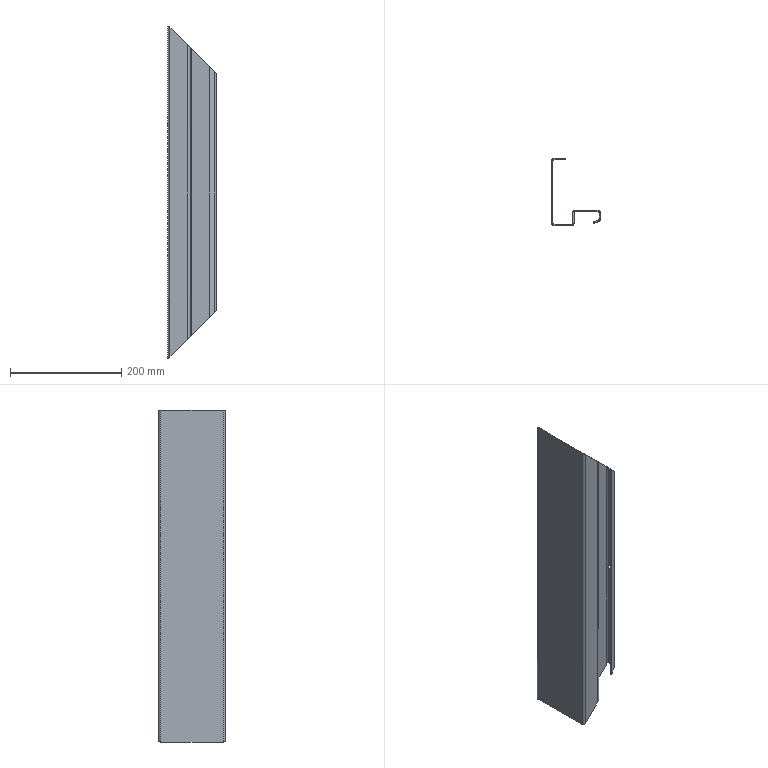Part | STEP file | 750038409 | 1 solid | 58 faces | box 87 x 120 x 596 mm | volume 299242 mm3 | plane 30 | cylinder 15 | spline 13 | commonest cylinder face diameters 4 x6 8 x6 11 x3